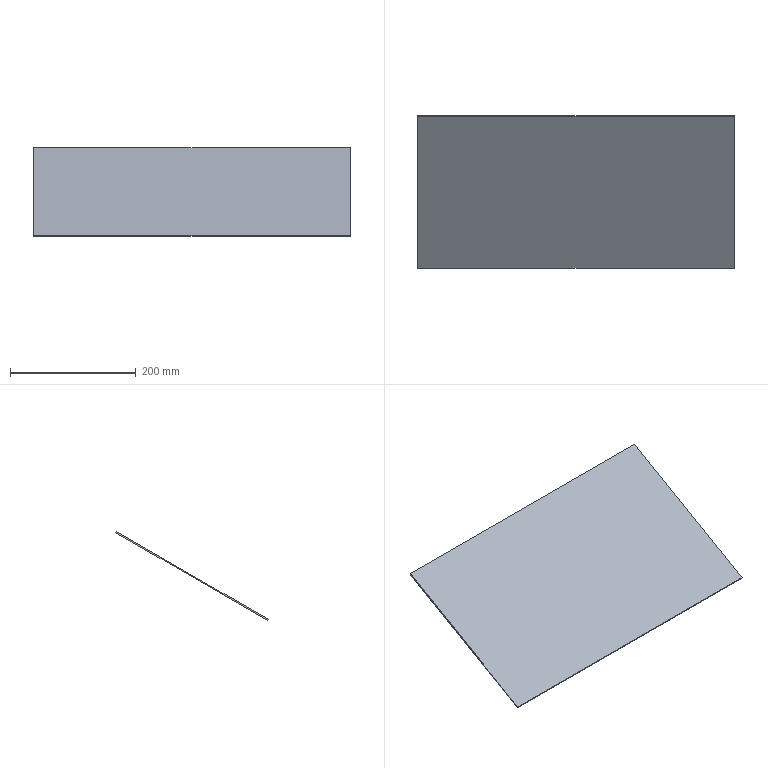Part | NX | features solid 2 | 1 solid | 6 faces | box 505 x 243.026 x 141.466 mm | volume 282262 mm3 | plane 6
STEP:
#1=CARTESIAN_POINT('',(15.,-367.603,-198.002));
#2=VERTEX_POINT('',#1);
#3=CARTESIAN_POINT('',(15.,-125.577,-58.268));
#4=VERTEX_POINT('',#3);
#5=CARTESIAN_POINT('',(15.,-271.,-142.228));
#6=DIRECTION('',(0.,0.866,0.5));
#7=VECTOR('',#6,1000.);
#8=LINE('',#5,#7);
#9=EDGE_CURVE('',#2,#4,#8,.T.);
#10=ORIENTED_EDGE('',*,*,#9,.T.);
#11=CARTESIAN_POINT('',(15.,-124.577,-60.));
#12=VERTEX_POINT('',#11);
#13=CARTESIAN_POINT('',(15.,-124.577,-60.));
#14=DIRECTION('',(0.,-0.5,0.866));
#15=VECTOR('',#14,1000.);
#16=LINE('',#13,#15);
#17=EDGE_CURVE('',#12,#4,#16,.T.);
#18=ORIENTED_EDGE('',*,*,#17,.F.);
#19=CARTESIAN_POINT('',(15.,-366.603,-199.734));
#20=VERTEX_POINT('',#19);
#21=CARTESIAN_POINT('',(15.,-270.,-143.96));
#22=DIRECTION('',(0.,0.866,0.5));
#23=VECTOR('',#22,1000.);
#24=LINE('',#21,#23);
#25=EDGE_CURVE('',#20,#12,#24,.T.);
#26=ORIENTED_EDGE('',*,*,#25,.F.);
#27=CARTESIAN_POINT('',(15.,-366.603,-199.734));
#28=DIRECTION('',(0.,-0.5,0.866));
#29=VECTOR('',#28,1000.);
#30=LINE('',#27,#29);
#31=EDGE_CURVE('',#20,#2,#30,.T.);
#32=ORIENTED_EDGE('',*,*,#31,.T.);
#33=EDGE_LOOP('',(#10,#18,#26,#32));
#34=FACE_BOUND('',#33,.T.);
#35=CARTESIAN_POINT('',(15.,-270.,-143.96));
#36=DIRECTION('',(1.,0.,0.));
#37=DIRECTION('',(0.,0.,-1.));
#38=AXIS2_PLACEMENT_3D('',#35,#36,#37);
#39=PLANE('',#38);
#40=ADVANCED_FACE('',(#34),#39,.F.);
#41=CARTESIAN_POINT('',(520.,-367.603,-198.002));
#42=VERTEX_POINT('',#41);
#43=CARTESIAN_POINT('',(230.,-367.603,-198.002));
#44=DIRECTION('',(-1.,0.,0.));
#45=VECTOR('',#44,1000.);
#46=LINE('',#43,#45);
#47=EDGE_CURVE('',#42,#2,#46,.T.);
#48=ORIENTED_EDGE('',*,*,#47,.T.);
#49=ORIENTED_EDGE('',*,*,#31,.F.);
#50=CARTESIAN_POINT('',(520.,-366.603,-199.734));
#51=VERTEX_POINT('',#50);
#52=CARTESIAN_POINT('',(230.,-366.603,-199.734));
#53=DIRECTION('',(-1.,0.,0.));
#54=VECTOR('',#53,1000.);
#55=LINE('',#52,#54);
#56=EDGE_CURVE('',#51,#20,#55,.T.);
#57=ORIENTED_EDGE('',*,*,#56,.F.);
#58=CARTESIAN_POINT('',(520.,-366.603,-199.734));
#59=DIRECTION('',(0.,-0.5,0.866));
#60=VECTOR('',#59,1000.);
#61=LINE('',#58,#60);
#62=EDGE_CURVE('',#51,#42,#61,.T.);
#63=ORIENTED_EDGE('',*,*,#62,.T.);
#64=EDGE_LOOP('',(#48,#49,#57,#63));
#65=FACE_BOUND('',#64,.T.);
#66=CARTESIAN_POINT('',(-690.,-366.603,-199.734));
#67=DIRECTION('',(0.,0.866,0.5));
#68=DIRECTION('',(0.,-0.5,0.866));
#69=AXIS2_PLACEMENT_3D('',#66,#67,#68);
#70=PLANE('',#69);
#71=ADVANCED_FACE('',(#65),#70,.F.);
#72=CARTESIAN_POINT('',(520.,-125.577,-58.268));
#73=VERTEX_POINT('',#72);
#74=CARTESIAN_POINT('',(520.,82.946,62.122));
#75=DIRECTION('',(0.,-0.866,-0.5));
#76=VECTOR('',#75,1000.);
#77=LINE('',#74,#76);
#78=EDGE_CURVE('',#42,#73,#77,.F.);
#79=ORIENTED_EDGE('',*,*,#78,.F.);
#80=ORIENTED_EDGE('',*,*,#62,.F.);
#81=CARTESIAN_POINT('',(520.,-124.577,-60.));
#82=VERTEX_POINT('',#81);
#83=CARTESIAN_POINT('',(520.,83.946,60.39));
#84=DIRECTION('',(0.,-0.866,-0.5));
#85=VECTOR('',#84,1000.);
#86=LINE('',#83,#85);
#87=EDGE_CURVE('',#51,#82,#86,.F.);
#88=ORIENTED_EDGE('',*,*,#87,.T.);
#89=CARTESIAN_POINT('',(520.,-124.577,-60.));
#90=DIRECTION('',(0.,-0.5,0.866));
#91=VECTOR('',#90,1000.);
#92=LINE('',#89,#91);
#93=EDGE_CURVE('',#82,#73,#92,.T.);
#94=ORIENTED_EDGE('',*,*,#93,.T.);
#95=EDGE_LOOP('',(#79,#80,#88,#94));
#96=FACE_BOUND('',#95,.T.);
#97=CARTESIAN_POINT('',(520.,83.946,60.39));
#98=DIRECTION('',(1.,0.,0.));
#99=DIRECTION('',(0.,0.,-1.));
#100=AXIS2_PLACEMENT_3D('',#97,#98,#99);
#101=PLANE('',#100);
#102=ADVANCED_FACE('',(#96),#101,.T.);
#103=CARTESIAN_POINT('',(230.,-125.577,-58.268));
#104=DIRECTION('',(-1.,0.,0.));
#105=VECTOR('',#104,1000.);
#106=LINE('',#103,#105);
#107=EDGE_CURVE('',#73,#4,#106,.T.);
#108=ORIENTED_EDGE('',*,*,#107,.F.);
#109=ORIENTED_EDGE('',*,*,#93,.F.);
#110=CARTESIAN_POINT('',(230.,-124.577,-60.));
#111=DIRECTION('',(-1.,0.,0.));
#112=VECTOR('',#111,1000.);
#113=LINE('',#110,#112);
#114=EDGE_CURVE('',#82,#12,#113,.T.);
#115=ORIENTED_EDGE('',*,*,#114,.T.);
#116=ORIENTED_EDGE('',*,*,#17,.T.);
#117=EDGE_LOOP('',(#108,#109,#115,#116));
#118=FACE_BOUND('',#117,.T.);
#119=CARTESIAN_POINT('',(230.,-124.577,-60.));
#120=DIRECTION('',(0.,0.866,0.5));
#121=DIRECTION('',(0.,-0.5,0.866));
#122=AXIS2_PLACEMENT_3D('',#119,#120,#121);
#123=PLANE('',#122);
#124=ADVANCED_FACE('',(#118),#123,.T.);
#125=ORIENTED_EDGE('',*,*,#25,.T.);
#126=ORIENTED_EDGE('',*,*,#114,.F.);
#127=ORIENTED_EDGE('',*,*,#87,.F.);
#128=ORIENTED_EDGE('',*,*,#56,.T.);
#129=EDGE_LOOP('',(#125,#126,#127,#128));
#130=FACE_BOUND('',#129,.T.);
#131=CARTESIAN_POINT('',(230.,-270.,-143.96));
#132=DIRECTION('',(0.,-0.5,0.866));
#133=DIRECTION('',(0.,-0.866,-0.5));
#134=AXIS2_PLACEMENT_3D('',#131,#132,#133);
#135=PLANE('',#134);
#136=ADVANCED_FACE('',(#130),#135,.F.);
#137=ORIENTED_EDGE('',*,*,#9,.F.);
#138=ORIENTED_EDGE('',*,*,#47,.F.);
#139=ORIENTED_EDGE('',*,*,#78,.T.);
#140=ORIENTED_EDGE('',*,*,#107,.T.);
#141=EDGE_LOOP('',(#137,#138,#139,#140));
#142=FACE_BOUND('',#141,.T.);
#143=CARTESIAN_POINT('',(230.,-271.,-142.228));
#144=DIRECTION('',(0.,-0.5,0.866));
#145=DIRECTION('',(0.,-0.866,-0.5));
#146=AXIS2_PLACEMENT_3D('',#143,#144,#145);
#147=PLANE('',#146);
#148=ADVANCED_FACE('',(#142),#147,.T.);
#149=CLOSED_SHELL('',(#40,#71,#102,#124,#136,#148));
#150=MANIFOLD_SOLID_BREP('',#149);
#151=(LENGTH_UNIT()NAMED_UNIT(*)SI_UNIT(.MILLI.,.METRE.));
#152=UNCERTAINTY_MEASURE_WITH_UNIT(LENGTH_MEASURE(0.00001),#151,'','');
#153=(NAMED_UNIT(*)PLANE_ANGLE_UNIT()SI_UNIT($,.RADIAN.));
#154=(NAMED_UNIT(*)SI_UNIT($,.STERADIAN.)SOLID_ANGLE_UNIT());
#155=(GEOMETRIC_REPRESENTATION_CONTEXT(3)GLOBAL_UNCERTAINTY_ASSIGNED_CONTEXT((#152))GLOBAL_UNIT_ASSIGNED_CONTEXT((#151,#153,#154))REPRESENTATION_CONTEXT('',''));
#156=ADVANCED_BREP_SHAPE_REPRESENTATION('',(#150),#155);